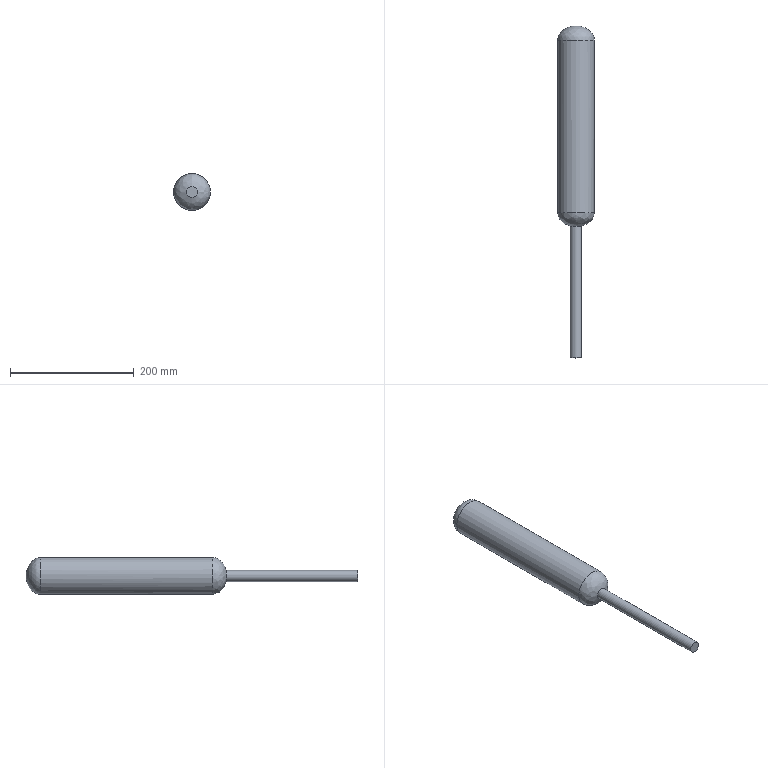Part | NX | features information lamp 2 | 1 solid | 5 faces | box 59.62 x 537.38 x 59.62 mm | volume 918566 mm3 | cylinder 2 | spline 2 | plane 1 | commonest cylinder face diameters 18 x1 59.62 x1
STEP:
#1=CARTESIAN_POINT('',(0.,-202.979,9.));
#2=VERTEX_POINT('',#1);
#3=CARTESIAN_POINT('',(0.,-202.979,0.));
#4=DIRECTION('',(0.,1.,0.));
#5=DIRECTION('',(0.,0.,1.));
#6=AXIS2_PLACEMENT_3D('',#3,#4,#5);
#7=CIRCLE('',#6,9.);
#8=EDGE_CURVE('',#2,#2,#7,.T.);
#9=ORIENTED_EDGE('',*,*,#8,.F.);
#10=EDGE_LOOP('',(#9));
#11=FACE_BOUND('',#10,.T.);
#12=CARTESIAN_POINT('',(9.,-202.979,0.));
#13=DIRECTION('',(0.,1.,0.));
#14=DIRECTION('',(0.,0.,1.));
#15=AXIS2_PLACEMENT_3D('',#12,#13,#14);
#16=PLANE('',#15);
#17=ADVANCED_FACE('',(#11),#16,.F.);
#18=ORIENTED_EDGE('',*,*,#8,.T.);
#19=EDGE_LOOP('',(#18));
#20=FACE_BOUND('',#19,.T.);
#21=CARTESIAN_POINT('',(0.,10.63,9.));
#22=VERTEX_POINT('',#21);
#23=CARTESIAN_POINT('',(0.,10.63,0.));
#24=DIRECTION('',(0.,1.,0.));
#25=DIRECTION('',(0.,0.,1.));
#26=AXIS2_PLACEMENT_3D('',#23,#24,#25);
#27=CIRCLE('',#26,9.);
#28=EDGE_CURVE('',#22,#22,#27,.T.);
#29=ORIENTED_EDGE('',*,*,#28,.F.);
#30=EDGE_LOOP('',(#29));
#31=FACE_BOUND('',#30,.T.);
#32=CARTESIAN_POINT('',(0.,311.547,0.));
#33=DIRECTION('',(0.,1.,0.));
#34=DIRECTION('',(0.,0.,1.));
#35=AXIS2_PLACEMENT_3D('',#32,#33,#34);
#36=CYLINDRICAL_SURFACE('',#35,9.);
#37=ADVANCED_FACE('',(#20,#31),#36,.T.);
#38=CARTESIAN_POINT('',(0.,32.418,29.81));
#39=VERTEX_POINT('',#38);
#40=CARTESIAN_POINT('',(0.,32.418,0.));
#41=DIRECTION('',(0.,1.,0.));
#42=DIRECTION('',(0.,0.,1.));
#43=AXIS2_PLACEMENT_3D('',#40,#41,#42);
#44=CIRCLE('',#43,29.81);
#45=EDGE_CURVE('',#39,#39,#44,.T.);
#46=ORIENTED_EDGE('',*,*,#45,.F.);
#47=EDGE_LOOP('',(#46));
#48=FACE_BOUND('',#47,.T.);
#49=ORIENTED_EDGE('',*,*,#28,.T.);
#50=EDGE_LOOP('',(#49));
#51=FACE_BOUND('',#50,.T.);
#52=CARTESIAN_POINT('',(29.81,32.418,0.));
#53=CARTESIAN_POINT('',(29.81,32.418,-59.62));
#54=CARTESIAN_POINT('',(-29.81,32.418,-59.62));
#55=CARTESIAN_POINT('',(-29.81,32.418,0.));
#56=CARTESIAN_POINT('',(-29.81,32.418,59.62));
#57=CARTESIAN_POINT('',(29.81,32.418,59.62));
#58=CARTESIAN_POINT('',(29.81,32.418,0.));
#59=CARTESIAN_POINT('',(29.81,21.261,0.));
#60=CARTESIAN_POINT('',(29.81,21.261,-59.62));
#61=CARTESIAN_POINT('',(-29.81,21.261,-59.62));
#62=CARTESIAN_POINT('',(-29.81,21.261,0.));
#63=CARTESIAN_POINT('',(-29.81,21.261,59.62));
#64=CARTESIAN_POINT('',(29.81,21.261,59.62));
#65=CARTESIAN_POINT('',(29.81,21.261,0.));
#66=CARTESIAN_POINT('',(20.77,13.488,0.));
#67=CARTESIAN_POINT('',(20.77,13.488,-41.539));
#68=CARTESIAN_POINT('',(-20.77,13.488,-41.539));
#69=CARTESIAN_POINT('',(-20.77,13.488,0.));
#70=CARTESIAN_POINT('',(-20.77,13.488,41.539));
#71=CARTESIAN_POINT('',(20.77,13.488,41.539));
#72=CARTESIAN_POINT('',(20.77,13.488,0.));
#73=CARTESIAN_POINT('',(9.,10.63,0.));
#74=CARTESIAN_POINT('',(9.,10.63,-18.));
#75=CARTESIAN_POINT('',(-9.,10.63,-18.));
#76=CARTESIAN_POINT('',(-9.,10.63,0.));
#77=CARTESIAN_POINT('',(-9.,10.63,18.));
#78=CARTESIAN_POINT('',(9.,10.63,18.));
#79=CARTESIAN_POINT('',(9.,10.63,0.));
#80=(BOUNDED_SURFACE()B_SPLINE_SURFACE(3,3,((#52,#53,#54,#55,#56,#57,#58),(#59,#60,#61,#62,#63,#64,#65),(#66,#67,#68,#69,#70,#71,#72),(#73,#74,#75,#76,#77,#78,#79)),.SURF_OF_REVOLUTION.,.F.,.T.,.F.)B_SPLINE_SURFACE_WITH_KNOTS((4,4),(1,3,3,3,1),(0.5,0.8661),(-0.5,0.,0.5,1.,1.5),.PIECEWISE_BEZIER_KNOTS.)GEOMETRIC_REPRESENTATION_ITEM()RATIONAL_B_SPLINE_SURFACE(((0.5,0.1667,0.1667,0.5,0.1667,0.1667,0.5),(0.5,0.1667,0.1667,0.5,0.1667,0.1667,0.5),(0.5894,0.1965,0.1965,0.5894,0.1965,0.1965,0.5894),(0.7681,0.256,0.256,0.7681,0.256,0.256,0.7681)))REPRESENTATION_ITEM('')SURFACE());
#81=ADVANCED_FACE('',(#48,#51),#80,.T.);
#82=CARTESIAN_POINT('',(0.,334.401,0.));
#83=VERTEX_POINT('',#82);
#84=VERTEX_LOOP('',#83);
#85=FACE_BOUND('',#84,.T.);
#86=CARTESIAN_POINT('',(0.,311.547,29.81));
#87=VERTEX_POINT('',#86);
#88=CARTESIAN_POINT('',(0.,311.547,0.));
#89=DIRECTION('',(0.,1.,0.));
#90=DIRECTION('',(0.,0.,1.));
#91=AXIS2_PLACEMENT_3D('',#88,#89,#90);
#92=CIRCLE('',#91,29.81);
#93=EDGE_CURVE('',#87,#87,#92,.F.);
#94=ORIENTED_EDGE('',*,*,#93,.F.);
#95=EDGE_LOOP('',(#94));
#96=FACE_BOUND('',#95,.T.);
#97=CARTESIAN_POINT('',(0.,334.401,0.));
#98=CARTESIAN_POINT('',(0.,334.401,0.));
#99=CARTESIAN_POINT('',(0.,334.401,0.));
#100=CARTESIAN_POINT('',(0.,334.401,0.));
#101=CARTESIAN_POINT('',(0.,334.401,0.));
#102=CARTESIAN_POINT('',(0.,334.401,0.));
#103=CARTESIAN_POINT('',(0.,334.401,0.));
#104=CARTESIAN_POINT('',(14.905,334.401,0.));
#105=CARTESIAN_POINT('',(14.905,334.401,-29.81));
#106=CARTESIAN_POINT('',(-14.905,334.401,-29.81));
#107=CARTESIAN_POINT('',(-14.905,334.401,0.));
#108=CARTESIAN_POINT('',(-14.905,334.401,29.81));
#109=CARTESIAN_POINT('',(14.905,334.401,29.81));
#110=CARTESIAN_POINT('',(14.905,334.401,0.));
#111=CARTESIAN_POINT('',(29.81,326.783,0.));
#112=CARTESIAN_POINT('',(29.81,326.783,-59.62));
#113=CARTESIAN_POINT('',(-29.81,326.783,-59.62));
#114=CARTESIAN_POINT('',(-29.81,326.783,0.));
#115=CARTESIAN_POINT('',(-29.81,326.783,59.62));
#116=CARTESIAN_POINT('',(29.81,326.783,59.62));
#117=CARTESIAN_POINT('',(29.81,326.783,0.));
#118=CARTESIAN_POINT('',(29.81,311.547,0.));
#119=CARTESIAN_POINT('',(29.81,311.547,-59.62));
#120=CARTESIAN_POINT('',(-29.81,311.547,-59.62));
#121=CARTESIAN_POINT('',(-29.81,311.547,0.));
#122=CARTESIAN_POINT('',(-29.81,311.547,59.62));
#123=CARTESIAN_POINT('',(29.81,311.547,59.62));
#124=CARTESIAN_POINT('',(29.81,311.547,0.));
#125=(BOUNDED_SURFACE()B_SPLINE_SURFACE(3,3,((#97,#98,#99,#100,#101,#102,#103),(#104,#105,#106,#107,#108,#109,#110),(#111,#112,#113,#114,#115,#116,#117),(#118,#119,#120,#121,#122,#123,#124)),.SURF_OF_REVOLUTION.,.F.,.T.,.F.)B_SPLINE_SURFACE_WITH_KNOTS((4,4),(1,3,3,3,1),(0.,0.5),(-0.5,0.,0.5,1.,1.5),.PIECEWISE_BEZIER_KNOTS.)GEOMETRIC_REPRESENTATION_ITEM()RATIONAL_B_SPLINE_SURFACE(((1.,0.3333,0.3333,1.,0.3333,0.3333,1.),(0.6667,0.2222,0.2222,0.6667,0.2222,0.2222,0.6667),(0.5,0.1667,0.1667,0.5,0.1667,0.1667,0.5),(0.5,0.1667,0.1667,0.5,0.1667,0.1667,0.5)))REPRESENTATION_ITEM('')SURFACE());
#126=ADVANCED_FACE('',(#85,#96),#125,.T.);
#127=ORIENTED_EDGE('',*,*,#45,.T.);
#128=EDGE_LOOP('',(#127));
#129=FACE_BOUND('',#128,.T.);
#130=ORIENTED_EDGE('',*,*,#93,.T.);
#131=EDGE_LOOP('',(#130));
#132=FACE_BOUND('',#131,.T.);
#133=CARTESIAN_POINT('',(0.,311.547,0.));
#134=DIRECTION('',(0.,1.,0.));
#135=DIRECTION('',(0.,0.,1.));
#136=AXIS2_PLACEMENT_3D('',#133,#134,#135);
#137=CYLINDRICAL_SURFACE('',#136,29.81);
#138=ADVANCED_FACE('',(#129,#132),#137,.T.);
#139=CLOSED_SHELL('',(#17,#37,#81,#126,#138));
#140=MANIFOLD_SOLID_BREP('',#139);
#141=(LENGTH_UNIT()NAMED_UNIT(*)SI_UNIT(.MILLI.,.METRE.));
#142=UNCERTAINTY_MEASURE_WITH_UNIT(LENGTH_MEASURE(0.00001),#141,'','');
#143=(NAMED_UNIT(*)PLANE_ANGLE_UNIT()SI_UNIT($,.RADIAN.));
#144=(NAMED_UNIT(*)SI_UNIT($,.STERADIAN.)SOLID_ANGLE_UNIT());
#145=(GEOMETRIC_REPRESENTATION_CONTEXT(3)GLOBAL_UNCERTAINTY_ASSIGNED_CONTEXT((#142))GLOBAL_UNIT_ASSIGNED_CONTEXT((#141,#143,#144))REPRESENTATION_CONTEXT('',''));
#146=ADVANCED_BREP_SHAPE_REPRESENTATION('',(#140),#145);